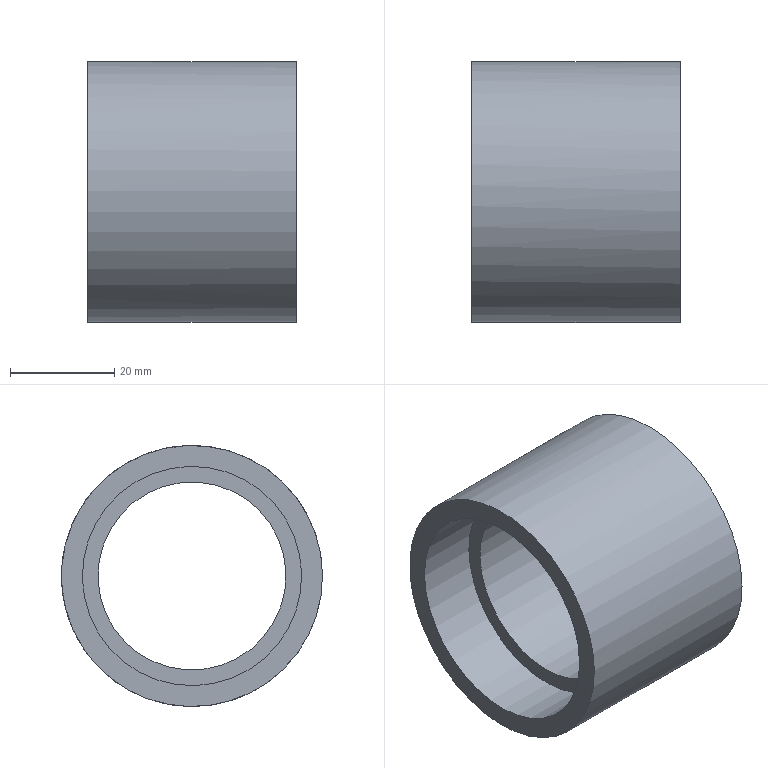Part | NX | features _-17204000 2 | 1 solid | 8 faces | box 40 x 50 x 50 mm | volume 29003 mm3 | plane 4 | cylinder 4 | commonest cylinder face diameters 42 x2 36 x1 50 x1
STEP:
#1=CARTESIAN_POINT('',(-15.5,-243.005,-692.818));
#2=VERTEX_POINT('',#1);
#3=CARTESIAN_POINT('',(-15.5,-260.8,-695.529));
#4=DIRECTION('',(1.,0.,0.));
#5=DIRECTION('',(0.,0.9886,0.1507));
#6=AXIS2_PLACEMENT_3D('',#3,#4,#5);
#7=CIRCLE('',#6,18.);
#8=EDGE_CURVE('',#2,#2,#7,.T.);
#9=ORIENTED_EDGE('',*,*,#8,.T.);
#10=EDGE_LOOP('',(#9));
#11=FACE_BOUND('',#10,.T.);
#12=CARTESIAN_POINT('',(-15.5,-240.04,-692.366));
#13=VERTEX_POINT('',#12);
#14=CARTESIAN_POINT('',(-15.5,-260.8,-695.529));
#15=DIRECTION('',(-1.,0.,0.));
#16=DIRECTION('',(0.,0.9886,0.1507));
#17=AXIS2_PLACEMENT_3D('',#14,#15,#16);
#18=CIRCLE('',#17,21.);
#19=EDGE_CURVE('',#13,#13,#18,.T.);
#20=ORIENTED_EDGE('',*,*,#19,.T.);
#21=EDGE_LOOP('',(#20));
#22=FACE_BOUND('',#21,.T.);
#23=CARTESIAN_POINT('',(-15.5,-260.8,-695.529));
#24=DIRECTION('',(-1.,0.,0.));
#25=DIRECTION('',(0.,0.9886,0.1507));
#26=AXIS2_PLACEMENT_3D('',#23,#24,#25);
#27=PLANE('',#26);
#28=ADVANCED_FACE('',(#11,#22),#27,.T.);
#29=ORIENTED_EDGE('',*,*,#19,.F.);
#30=EDGE_LOOP('',(#29));
#31=FACE_BOUND('',#30,.T.);
#32=CARTESIAN_POINT('',(-27.5,-281.56,-698.693));
#33=VERTEX_POINT('',#32);
#34=CARTESIAN_POINT('',(-27.5,-260.8,-695.529));
#35=DIRECTION('',(1.,0.,0.));
#36=DIRECTION('',(0.,-0.9886,-0.1507));
#37=AXIS2_PLACEMENT_3D('',#34,#35,#36);
#38=CIRCLE('',#37,21.);
#39=EDGE_CURVE('',#33,#33,#38,.T.);
#40=ORIENTED_EDGE('',*,*,#39,.F.);
#41=EDGE_LOOP('',(#40));
#42=FACE_BOUND('',#41,.T.);
#43=CARTESIAN_POINT('',(-15.5,-260.8,-695.529));
#44=DIRECTION('',(-1.,0.,0.));
#45=DIRECTION('',(0.,0.9886,0.1507));
#46=AXIS2_PLACEMENT_3D('',#43,#44,#45);
#47=CYLINDRICAL_SURFACE('',#46,21.);
#48=ADVANCED_FACE('',(#31,#42),#47,.F.);
#49=ORIENTED_EDGE('',*,*,#39,.T.);
#50=EDGE_LOOP('',(#49));
#51=FACE_BOUND('',#50,.T.);
#52=CARTESIAN_POINT('',(-27.5,-285.515,-699.296));
#53=VERTEX_POINT('',#52);
#54=CARTESIAN_POINT('',(-27.5,-260.8,-695.529));
#55=DIRECTION('',(-1.,0.,0.));
#56=DIRECTION('',(0.,-0.9886,-0.1507));
#57=AXIS2_PLACEMENT_3D('',#54,#55,#56);
#58=CIRCLE('',#57,25.);
#59=EDGE_CURVE('',#53,#53,#58,.T.);
#60=ORIENTED_EDGE('',*,*,#59,.T.);
#61=EDGE_LOOP('',(#60));
#62=FACE_BOUND('',#61,.T.);
#63=CARTESIAN_POINT('',(-27.5,-260.8,-695.529));
#64=DIRECTION('',(-1.,0.,0.));
#65=DIRECTION('',(0.,0.9886,0.1507));
#66=AXIS2_PLACEMENT_3D('',#63,#64,#65);
#67=PLANE('',#66);
#68=ADVANCED_FACE('',(#51,#62),#67,.T.);
#69=CARTESIAN_POINT('',(12.5,-236.085,-691.763));
#70=VERTEX_POINT('',#69);
#71=CARTESIAN_POINT('',(12.5,-260.8,-695.529));
#72=DIRECTION('',(1.,0.,0.));
#73=DIRECTION('',(0.,0.9886,0.1507));
#74=AXIS2_PLACEMENT_3D('',#71,#72,#73);
#75=CIRCLE('',#74,25.);
#76=EDGE_CURVE('',#70,#70,#75,.T.);
#77=ORIENTED_EDGE('',*,*,#76,.F.);
#78=EDGE_LOOP('',(#77));
#79=FACE_BOUND('',#78,.T.);
#80=ORIENTED_EDGE('',*,*,#59,.F.);
#81=EDGE_LOOP('',(#80));
#82=FACE_BOUND('',#81,.T.);
#83=CARTESIAN_POINT('',(-27.5,-260.8,-695.529));
#84=DIRECTION('',(1.,0.,0.));
#85=DIRECTION('',(0.,-0.9886,-0.1507));
#86=AXIS2_PLACEMENT_3D('',#83,#84,#85);
#87=CYLINDRICAL_SURFACE('',#86,25.);
#88=ADVANCED_FACE('',(#79,#82),#87,.T.);
#89=CARTESIAN_POINT('',(12.5,-281.56,-698.693));
#90=VERTEX_POINT('',#89);
#91=CARTESIAN_POINT('',(12.5,-260.8,-695.529));
#92=DIRECTION('',(-1.,0.,0.));
#93=DIRECTION('',(0.,-0.9886,-0.1507));
#94=AXIS2_PLACEMENT_3D('',#91,#92,#93);
#95=CIRCLE('',#94,21.);
#96=EDGE_CURVE('',#90,#90,#95,.T.);
#97=ORIENTED_EDGE('',*,*,#96,.T.);
#98=EDGE_LOOP('',(#97));
#99=FACE_BOUND('',#98,.T.);
#100=ORIENTED_EDGE('',*,*,#76,.T.);
#101=EDGE_LOOP('',(#100));
#102=FACE_BOUND('',#101,.T.);
#103=CARTESIAN_POINT('',(12.5,-260.8,-695.529));
#104=DIRECTION('',(-1.,0.,0.));
#105=DIRECTION('',(0.,0.9886,0.1507));
#106=AXIS2_PLACEMENT_3D('',#103,#104,#105);
#107=PLANE('',#106);
#108=ADVANCED_FACE('',(#99,#102),#107,.F.);
#109=CARTESIAN_POINT('',(0.5,-240.04,-692.366));
#110=VERTEX_POINT('',#109);
#111=CARTESIAN_POINT('',(0.5,-260.8,-695.529));
#112=DIRECTION('',(1.,0.,0.));
#113=DIRECTION('',(0.,0.9886,0.1507));
#114=AXIS2_PLACEMENT_3D('',#111,#112,#113);
#115=CIRCLE('',#114,21.);
#116=EDGE_CURVE('',#110,#110,#115,.T.);
#117=ORIENTED_EDGE('',*,*,#116,.F.);
#118=EDGE_LOOP('',(#117));
#119=FACE_BOUND('',#118,.T.);
#120=ORIENTED_EDGE('',*,*,#96,.F.);
#121=EDGE_LOOP('',(#120));
#122=FACE_BOUND('',#121,.T.);
#123=CARTESIAN_POINT('',(0.5,-260.8,-695.529));
#124=DIRECTION('',(1.,0.,0.));
#125=DIRECTION('',(0.,-0.9886,-0.1507));
#126=AXIS2_PLACEMENT_3D('',#123,#124,#125);
#127=CYLINDRICAL_SURFACE('',#126,21.);
#128=ADVANCED_FACE('',(#119,#122),#127,.F.);
#129=CARTESIAN_POINT('',(0.5,-278.595,-698.241));
#130=VERTEX_POINT('',#129);
#131=CARTESIAN_POINT('',(0.5,-260.8,-695.529));
#132=DIRECTION('',(-1.,0.,0.));
#133=DIRECTION('',(0.,-0.9886,-0.1507));
#134=AXIS2_PLACEMENT_3D('',#131,#132,#133);
#135=CIRCLE('',#134,18.);
#136=EDGE_CURVE('',#130,#130,#135,.T.);
#137=ORIENTED_EDGE('',*,*,#136,.T.);
#138=EDGE_LOOP('',(#137));
#139=FACE_BOUND('',#138,.T.);
#140=ORIENTED_EDGE('',*,*,#116,.T.);
#141=EDGE_LOOP('',(#140));
#142=FACE_BOUND('',#141,.T.);
#143=CARTESIAN_POINT('',(0.5,-260.8,-695.529));
#144=DIRECTION('',(1.,0.,0.));
#145=DIRECTION('',(0.,0.9886,0.1507));
#146=AXIS2_PLACEMENT_3D('',#143,#144,#145);
#147=PLANE('',#146);
#148=ADVANCED_FACE('',(#139,#142),#147,.T.);
#149=ORIENTED_EDGE('',*,*,#136,.F.);
#150=EDGE_LOOP('',(#149));
#151=FACE_BOUND('',#150,.T.);
#152=ORIENTED_EDGE('',*,*,#8,.F.);
#153=EDGE_LOOP('',(#152));
#154=FACE_BOUND('',#153,.T.);
#155=CARTESIAN_POINT('',(12.5,-260.8,-695.529));
#156=DIRECTION('',(-1.,0.,0.));
#157=DIRECTION('',(0.,0.9886,0.1507));
#158=AXIS2_PLACEMENT_3D('',#155,#156,#157);
#159=CYLINDRICAL_SURFACE('',#158,18.);
#160=ADVANCED_FACE('',(#151,#154),#159,.F.);
#161=CLOSED_SHELL('',(#28,#48,#68,#88,#108,#128,#148,#160));
#162=MANIFOLD_SOLID_BREP('',#161);
#163=(LENGTH_UNIT()NAMED_UNIT(*)SI_UNIT(.MILLI.,.METRE.));
#164=UNCERTAINTY_MEASURE_WITH_UNIT(LENGTH_MEASURE(0.00001),#163,'','');
#165=(NAMED_UNIT(*)PLANE_ANGLE_UNIT()SI_UNIT($,.RADIAN.));
#166=(NAMED_UNIT(*)SI_UNIT($,.STERADIAN.)SOLID_ANGLE_UNIT());
#167=(GEOMETRIC_REPRESENTATION_CONTEXT(3)GLOBAL_UNCERTAINTY_ASSIGNED_CONTEXT((#164))GLOBAL_UNIT_ASSIGNED_CONTEXT((#163,#165,#166))REPRESENTATION_CONTEXT('',''));
#168=ADVANCED_BREP_SHAPE_REPRESENTATION('',(#162),#167);